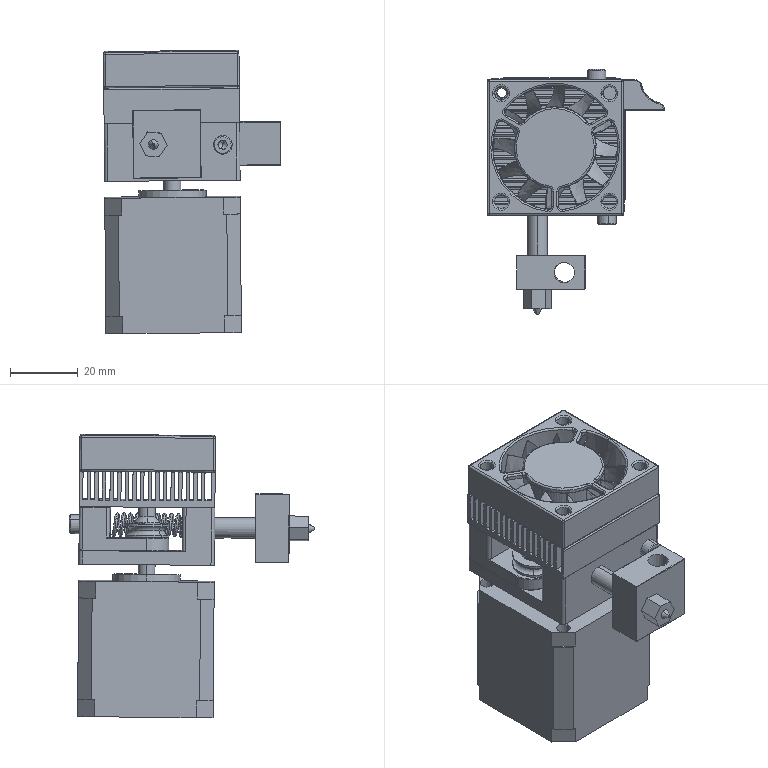Part | SolidWorks | 26 solids | 1028 faces | box 52.269 x 72.401 x 83.639 mm | volume 115279 mm3 | cylinder 390 | plane 372 | cone 116 | spline 74 | torus 66 | sphere 10 | commonest cylinder face diameters 1 x73 11 x42 4 x39 5 x32 24 x28 8 x26